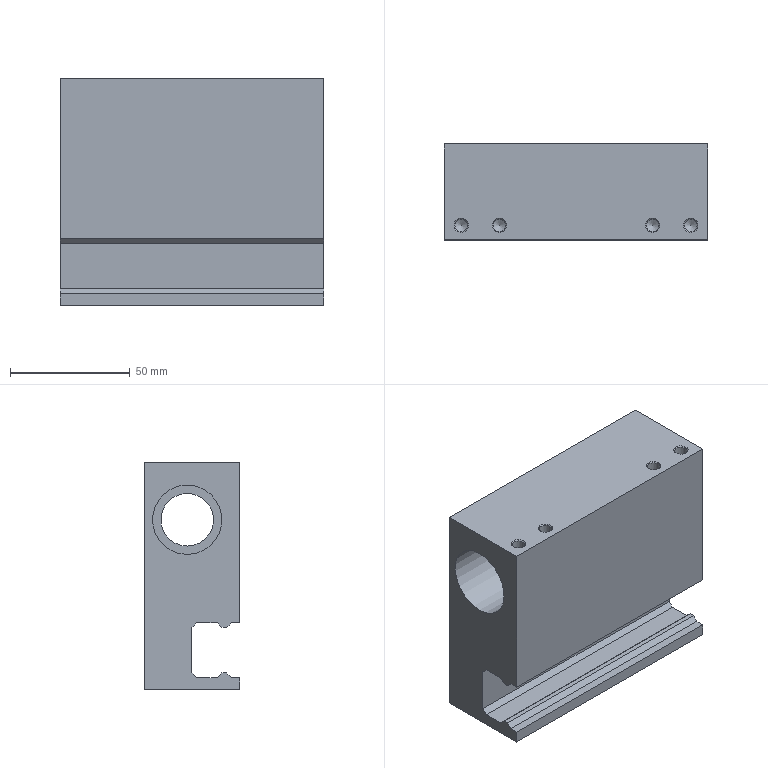Part | NX | features SIMPLE HOLE 10, SYMBOLIC_THREAD 9, DATUM_CSYS 5, HOLE PACKAGE 4, SKETCH 4, EXTRUDE 2, SUBTRACT 1 | 1 solid | 49 faces | box 110 x 40 x 95 mm | volume 307635 mm3 | plane 22 | cone 16 | cylinder 11 | commonest cylinder face diameters 5.2 x8 29 x2 22 x1
STEP:
#1=CARTESIAN_POINT('',(-55.,-3.5,11.5));
#2=VERTEX_POINT('',#1);
#3=CARTESIAN_POINT('',(55.,-3.5,11.5));
#4=VERTEX_POINT('',#3);
#5=CARTESIAN_POINT('',(55.,-3.5,11.5));
#6=DIRECTION('',(-1.,0.,0.));
#7=VECTOR('',#6,1000.);
#8=LINE('',#5,#7);
#9=EDGE_CURVE('',#2,#4,#8,.F.);
#10=ORIENTED_EDGE('',*,*,#9,.T.);
#11=CARTESIAN_POINT('',(55.,-3.5,78.5));
#12=VERTEX_POINT('',#11);
#13=CARTESIAN_POINT('',(55.,-3.5,78.5));
#14=DIRECTION('',(0.,0.,-1.));
#15=VECTOR('',#14,1000.);
#16=LINE('',#13,#15);
#17=EDGE_CURVE('',#12,#4,#16,.T.);
#18=ORIENTED_EDGE('',*,*,#17,.F.);
#19=CARTESIAN_POINT('',(-55.,-3.5,78.5));
#20=VERTEX_POINT('',#19);
#21=CARTESIAN_POINT('',(55.,-3.5,78.5));
#22=DIRECTION('',(-1.,0.,0.));
#23=VECTOR('',#22,1000.);
#24=LINE('',#21,#23);
#25=EDGE_CURVE('',#12,#20,#24,.T.);
#26=ORIENTED_EDGE('',*,*,#25,.T.);
#27=CARTESIAN_POINT('',(-55.,-3.5,78.5));
#28=DIRECTION('',(0.,0.,-1.));
#29=VECTOR('',#28,1000.);
#30=LINE('',#27,#29);
#31=EDGE_CURVE('',#20,#2,#30,.T.);
#32=ORIENTED_EDGE('',*,*,#31,.T.);
#33=EDGE_LOOP('',(#10,#18,#26,#32));
#34=FACE_BOUND('',#33,.T.);
#35=CARTESIAN_POINT('',(55.,-3.5,78.5));
#36=DIRECTION('',(0.,1.,0.));
#37=DIRECTION('',(0.,0.,1.));
#38=AXIS2_PLACEMENT_3D('',#35,#36,#37);
#39=PLANE('',#38);
#40=ADVANCED_FACE('',(#34),#39,.F.);
#41=CARTESIAN_POINT('',(55.,-3.5,-11.5));
#42=VERTEX_POINT('',#41);
#43=CARTESIAN_POINT('',(-55.,-3.5,-11.5));
#44=VERTEX_POINT('',#43);
#45=CARTESIAN_POINT('',(55.,-3.5,-11.5));
#46=DIRECTION('',(1.,0.,0.));
#47=VECTOR('',#46,1000.);
#48=LINE('',#45,#47);
#49=EDGE_CURVE('',#42,#44,#48,.F.);
#50=ORIENTED_EDGE('',*,*,#49,.T.);
#51=CARTESIAN_POINT('',(-55.,-3.5,-16.5));
#52=VERTEX_POINT('',#51);
#53=CARTESIAN_POINT('',(-55.,-3.5,78.5));
#54=DIRECTION('',(0.,0.,-1.));
#55=VECTOR('',#54,1000.);
#56=LINE('',#53,#55);
#57=EDGE_CURVE('',#44,#52,#56,.T.);
#58=ORIENTED_EDGE('',*,*,#57,.T.);
#59=CARTESIAN_POINT('',(55.,-3.5,-16.5));
#60=VERTEX_POINT('',#59);
#61=CARTESIAN_POINT('',(55.,-3.5,-16.5));
#62=DIRECTION('',(-1.,0.,0.));
#63=VECTOR('',#62,1000.);
#64=LINE('',#61,#63);
#65=EDGE_CURVE('',#60,#52,#64,.T.);
#66=ORIENTED_EDGE('',*,*,#65,.F.);
#67=CARTESIAN_POINT('',(55.,-3.5,78.5));
#68=DIRECTION('',(0.,0.,-1.));
#69=VECTOR('',#68,1000.);
#70=LINE('',#67,#69);
#71=EDGE_CURVE('',#42,#60,#70,.T.);
#72=ORIENTED_EDGE('',*,*,#71,.F.);
#73=EDGE_LOOP('',(#50,#58,#66,#72));
#74=FACE_BOUND('',#73,.T.);
#75=CARTESIAN_POINT('',(55.,-3.5,78.5));
#76=DIRECTION('',(0.,1.,0.));
#77=DIRECTION('',(0.,0.,1.));
#78=AXIS2_PLACEMENT_3D('',#75,#76,#77);
#79=PLANE('',#78);
#80=ADVANCED_FACE('',(#74),#79,.F.);
#81=CARTESIAN_POINT('',(55.,18.5,69.));
#82=VERTEX_POINT('',#81);
#83=CARTESIAN_POINT('',(55.,18.5,54.5));
#84=DIRECTION('',(-1.,0.,0.));
#85=DIRECTION('',(0.,0.,1.));
#86=AXIS2_PLACEMENT_3D('',#83,#84,#85);
#87=CIRCLE('',#86,14.5);
#88=EDGE_CURVE('',#82,#82,#87,.T.);
#89=ORIENTED_EDGE('',*,*,#88,.T.);
#90=EDGE_LOOP('',(#89));
#91=FACE_BOUND('',#90,.T.);
#92=ORIENTED_EDGE('',*,*,#17,.T.);
#93=CARTESIAN_POINT('',(55.,0.,11.5));
#94=VERTEX_POINT('',#93);
#95=CARTESIAN_POINT('',(55.,18.5,11.5));
#96=DIRECTION('',(0.,1.,0.));
#97=VECTOR('',#96,1000.);
#98=LINE('',#95,#97);
#99=EDGE_CURVE('',#94,#4,#98,.F.);
#100=ORIENTED_EDGE('',*,*,#99,.F.);
#101=CARTESIAN_POINT('',(55.,2.,9.5));
#102=VERTEX_POINT('',#101);
#103=CARTESIAN_POINT('',(55.,-12.25,23.75));
#104=DIRECTION('',(0.,0.7071,-0.7071));
#105=VECTOR('',#104,1000.);
#106=LINE('',#103,#105);
#107=EDGE_CURVE('',#102,#94,#106,.F.);
#108=ORIENTED_EDGE('',*,*,#107,.F.);
#109=CARTESIAN_POINT('',(55.,4.,9.5));
#110=VERTEX_POINT('',#109);
#111=CARTESIAN_POINT('',(55.,18.5,9.5));
#112=DIRECTION('',(0.,1.,0.));
#113=VECTOR('',#112,1000.);
#114=LINE('',#111,#113);
#115=EDGE_CURVE('',#110,#102,#114,.F.);
#116=ORIENTED_EDGE('',*,*,#115,.F.);
#117=CARTESIAN_POINT('',(55.,6.,11.5));
#118=VERTEX_POINT('',#117);
#119=CARTESIAN_POINT('',(55.,33.75,39.25));
#120=DIRECTION('',(0.,0.7071,0.7071));
#121=VECTOR('',#120,1000.);
#122=LINE('',#119,#121);
#123=EDGE_CURVE('',#118,#110,#122,.F.);
#124=ORIENTED_EDGE('',*,*,#123,.F.);
#125=CARTESIAN_POINT('',(55.,14.5,11.5));
#126=VERTEX_POINT('',#125);
#127=CARTESIAN_POINT('',(55.,18.5,11.5));
#128=DIRECTION('',(0.,1.,0.));
#129=VECTOR('',#128,1000.);
#130=LINE('',#127,#129);
#131=EDGE_CURVE('',#126,#118,#130,.F.);
#132=ORIENTED_EDGE('',*,*,#131,.F.);
#133=CARTESIAN_POINT('',(55.,16.5,9.5));
#134=VERTEX_POINT('',#133);
#135=CARTESIAN_POINT('',(55.,-5.,31.));
#136=DIRECTION('',(0.,0.7071,-0.7071));
#137=VECTOR('',#136,1000.);
#138=LINE('',#135,#137);
#139=EDGE_CURVE('',#134,#126,#138,.F.);
#140=ORIENTED_EDGE('',*,*,#139,.F.);
#141=CARTESIAN_POINT('',(55.,16.5,-9.5));
#142=VERTEX_POINT('',#141);
#143=CARTESIAN_POINT('',(55.,16.5,54.5));
#144=DIRECTION('',(0.,0.,-1.));
#145=VECTOR('',#144,1000.);
#146=LINE('',#143,#145);
#147=EDGE_CURVE('',#142,#134,#146,.F.);
#148=ORIENTED_EDGE('',*,*,#147,.F.);
#149=CARTESIAN_POINT('',(55.,14.5,-11.5));
#150=VERTEX_POINT('',#149);
#151=CARTESIAN_POINT('',(55.,49.5,23.5));
#152=DIRECTION('',(0.,-0.7071,-0.7071));
#153=VECTOR('',#152,1000.);
#154=LINE('',#151,#153);
#155=EDGE_CURVE('',#150,#142,#154,.F.);
#156=ORIENTED_EDGE('',*,*,#155,.F.);
#157=CARTESIAN_POINT('',(55.,6.,-11.5));
#158=VERTEX_POINT('',#157);
#159=CARTESIAN_POINT('',(55.,18.5,-11.5));
#160=DIRECTION('',(0.,-1.,0.));
#161=VECTOR('',#160,1000.);
#162=LINE('',#159,#161);
#163=EDGE_CURVE('',#158,#150,#162,.F.);
#164=ORIENTED_EDGE('',*,*,#163,.F.);
#165=CARTESIAN_POINT('',(55.,4.,-9.5));
#166=VERTEX_POINT('',#165);
#167=CARTESIAN_POINT('',(55.,-20.75,15.25));
#168=DIRECTION('',(0.,-0.7071,0.7071));
#169=VECTOR('',#168,1000.);
#170=LINE('',#167,#169);
#171=EDGE_CURVE('',#166,#158,#170,.F.);
#172=ORIENTED_EDGE('',*,*,#171,.F.);
#173=CARTESIAN_POINT('',(55.,2.,-9.5));
#174=VERTEX_POINT('',#173);
#175=CARTESIAN_POINT('',(55.,18.5,-9.5));
#176=DIRECTION('',(0.,-1.,0.));
#177=VECTOR('',#176,1000.);
#178=LINE('',#175,#177);
#179=EDGE_CURVE('',#174,#166,#178,.F.);
#180=ORIENTED_EDGE('',*,*,#179,.F.);
#181=CARTESIAN_POINT('',(55.,0.,-11.5));
#182=VERTEX_POINT('',#181);
#183=CARTESIAN_POINT('',(55.,42.25,30.75));
#184=DIRECTION('',(0.,-0.7071,-0.7071));
#185=VECTOR('',#184,1000.);
#186=LINE('',#183,#185);
#187=EDGE_CURVE('',#182,#174,#186,.F.);
#188=ORIENTED_EDGE('',*,*,#187,.F.);
#189=CARTESIAN_POINT('',(55.,18.5,-11.5));
#190=DIRECTION('',(0.,-1.,0.));
#191=VECTOR('',#190,1000.);
#192=LINE('',#189,#191);
#193=EDGE_CURVE('',#42,#182,#192,.F.);
#194=ORIENTED_EDGE('',*,*,#193,.F.);
#195=ORIENTED_EDGE('',*,*,#71,.T.);
#196=CARTESIAN_POINT('',(55.,36.5,-16.5));
#197=VERTEX_POINT('',#196);
#198=CARTESIAN_POINT('',(55.,-3.5,-16.5));
#199=DIRECTION('',(0.,1.,0.));
#200=VECTOR('',#199,1000.);
#201=LINE('',#198,#200);
#202=EDGE_CURVE('',#60,#197,#201,.T.);
#203=ORIENTED_EDGE('',*,*,#202,.T.);
#204=CARTESIAN_POINT('',(55.,36.5,78.5));
#205=VERTEX_POINT('',#204);
#206=CARTESIAN_POINT('',(55.,36.5,-16.5));
#207=DIRECTION('',(0.,0.,1.));
#208=VECTOR('',#207,1000.);
#209=LINE('',#206,#208);
#210=EDGE_CURVE('',#197,#205,#209,.T.);
#211=ORIENTED_EDGE('',*,*,#210,.T.);
#212=CARTESIAN_POINT('',(55.,36.5,78.5));
#213=DIRECTION('',(0.,-1.,0.));
#214=VECTOR('',#213,1000.);
#215=LINE('',#212,#214);
#216=EDGE_CURVE('',#205,#12,#215,.T.);
#217=ORIENTED_EDGE('',*,*,#216,.T.);
#218=EDGE_LOOP('',(#92,#100,#108,#116,#124,#132,#140,#148,#156,#164,#172,#180,#188,#194,#195,#203,#211,#217));
#219=FACE_BOUND('',#218,.T.);
#220=CARTESIAN_POINT('',(55.,18.5,54.5));
#221=DIRECTION('',(1.,0.,0.));
#222=DIRECTION('',(0.,0.,-1.));
#223=AXIS2_PLACEMENT_3D('',#220,#221,#222);
#224=PLANE('',#223);
#225=ADVANCED_FACE('',(#91,#219),#224,.T.);
#226=CARTESIAN_POINT('',(-55.,18.5,40.));
#227=VERTEX_POINT('',#226);
#228=CARTESIAN_POINT('',(-55.,18.5,54.5));
#229=DIRECTION('',(1.,0.,0.));
#230=DIRECTION('',(0.,0.,-1.));
#231=AXIS2_PLACEMENT_3D('',#228,#229,#230);
#232=CIRCLE('',#231,14.5);
#233=EDGE_CURVE('',#227,#227,#232,.T.);
#234=ORIENTED_EDGE('',*,*,#233,.T.);
#235=EDGE_LOOP('',(#234));
#236=FACE_BOUND('',#235,.T.);
#237=CARTESIAN_POINT('',(-55.,0.,11.5));
#238=VERTEX_POINT('',#237);
#239=CARTESIAN_POINT('',(-55.,18.5,11.5));
#240=DIRECTION('',(0.,1.,0.));
#241=VECTOR('',#240,1000.);
#242=LINE('',#239,#241);
#243=EDGE_CURVE('',#238,#2,#242,.F.);
#244=ORIENTED_EDGE('',*,*,#243,.T.);
#245=ORIENTED_EDGE('',*,*,#31,.F.);
#246=CARTESIAN_POINT('',(-55.,36.5,78.5));
#247=VERTEX_POINT('',#246);
#248=CARTESIAN_POINT('',(-55.,36.5,78.5));
#249=DIRECTION('',(0.,-1.,0.));
#250=VECTOR('',#249,1000.);
#251=LINE('',#248,#250);
#252=EDGE_CURVE('',#247,#20,#251,.T.);
#253=ORIENTED_EDGE('',*,*,#252,.F.);
#254=CARTESIAN_POINT('',(-55.,36.5,-16.5));
#255=VERTEX_POINT('',#254);
#256=CARTESIAN_POINT('',(-55.,36.5,-16.5));
#257=DIRECTION('',(0.,0.,1.));
#258=VECTOR('',#257,1000.);
#259=LINE('',#256,#258);
#260=EDGE_CURVE('',#255,#247,#259,.T.);
#261=ORIENTED_EDGE('',*,*,#260,.F.);
#262=CARTESIAN_POINT('',(-55.,-3.5,-16.5));
#263=DIRECTION('',(0.,1.,0.));
#264=VECTOR('',#263,1000.);
#265=LINE('',#262,#264);
#266=EDGE_CURVE('',#52,#255,#265,.T.);
#267=ORIENTED_EDGE('',*,*,#266,.F.);
#268=ORIENTED_EDGE('',*,*,#57,.F.);
#269=CARTESIAN_POINT('',(-55.,0.,-11.5));
#270=VERTEX_POINT('',#269);
#271=CARTESIAN_POINT('',(-55.,18.5,-11.5));
#272=DIRECTION('',(0.,-1.,0.));
#273=VECTOR('',#272,1000.);
#274=LINE('',#271,#273);
#275=EDGE_CURVE('',#44,#270,#274,.F.);
#276=ORIENTED_EDGE('',*,*,#275,.T.);
#277=CARTESIAN_POINT('',(-55.,2.,-9.5));
#278=VERTEX_POINT('',#277);
#279=CARTESIAN_POINT('',(-55.,42.25,30.75));
#280=DIRECTION('',(0.,-0.7071,-0.7071));
#281=VECTOR('',#280,1000.);
#282=LINE('',#279,#281);
#283=EDGE_CURVE('',#270,#278,#282,.F.);
#284=ORIENTED_EDGE('',*,*,#283,.T.);
#285=CARTESIAN_POINT('',(-55.,4.,-9.5));
#286=VERTEX_POINT('',#285);
#287=CARTESIAN_POINT('',(-55.,18.5,-9.5));
#288=DIRECTION('',(0.,-1.,0.));
#289=VECTOR('',#288,1000.);
#290=LINE('',#287,#289);
#291=EDGE_CURVE('',#278,#286,#290,.F.);
#292=ORIENTED_EDGE('',*,*,#291,.T.);
#293=CARTESIAN_POINT('',(-55.,6.,-11.5));
#294=VERTEX_POINT('',#293);
#295=CARTESIAN_POINT('',(-55.,-20.75,15.25));
#296=DIRECTION('',(0.,-0.7071,0.7071));
#297=VECTOR('',#296,1000.);
#298=LINE('',#295,#297);
#299=EDGE_CURVE('',#286,#294,#298,.F.);
#300=ORIENTED_EDGE('',*,*,#299,.T.);
#301=CARTESIAN_POINT('',(-55.,14.5,-11.5));
#302=VERTEX_POINT('',#301);
#303=CARTESIAN_POINT('',(-55.,18.5,-11.5));
#304=DIRECTION('',(0.,-1.,0.));
#305=VECTOR('',#304,1000.);
#306=LINE('',#303,#305);
#307=EDGE_CURVE('',#294,#302,#306,.F.);
#308=ORIENTED_EDGE('',*,*,#307,.T.);
#309=CARTESIAN_POINT('',(-55.,16.5,-9.5));
#310=VERTEX_POINT('',#309);
#311=CARTESIAN_POINT('',(-55.,49.5,23.5));
#312=DIRECTION('',(0.,-0.7071,-0.7071));
#313=VECTOR('',#312,1000.);
#314=LINE('',#311,#313);
#315=EDGE_CURVE('',#302,#310,#314,.F.);
#316=ORIENTED_EDGE('',*,*,#315,.T.);
#317=CARTESIAN_POINT('',(-55.,16.5,9.5));
#318=VERTEX_POINT('',#317);
#319=CARTESIAN_POINT('',(-55.,16.5,54.5));
#320=DIRECTION('',(0.,0.,-1.));
#321=VECTOR('',#320,1000.);
#322=LINE('',#319,#321);
#323=EDGE_CURVE('',#310,#318,#322,.F.);
#324=ORIENTED_EDGE('',*,*,#323,.T.);
#325=CARTESIAN_POINT('',(-55.,14.5,11.5));
#326=VERTEX_POINT('',#325);
#327=CARTESIAN_POINT('',(-55.,-5.,31.));
#328=DIRECTION('',(0.,0.7071,-0.7071));
#329=VECTOR('',#328,1000.);
#330=LINE('',#327,#329);
#331=EDGE_CURVE('',#318,#326,#330,.F.);
#332=ORIENTED_EDGE('',*,*,#331,.T.);
#333=CARTESIAN_POINT('',(-55.,6.,11.5));
#334=VERTEX_POINT('',#333);
#335=CARTESIAN_POINT('',(-55.,18.5,11.5));
#336=DIRECTION('',(0.,1.,0.));
#337=VECTOR('',#336,1000.);
#338=LINE('',#335,#337);
#339=EDGE_CURVE('',#326,#334,#338,.F.);
#340=ORIENTED_EDGE('',*,*,#339,.T.);
#341=CARTESIAN_POINT('',(-55.,4.,9.5));
#342=VERTEX_POINT('',#341);
#343=CARTESIAN_POINT('',(-55.,33.75,39.25));
#344=DIRECTION('',(0.,0.7071,0.7071));
#345=VECTOR('',#344,1000.);
#346=LINE('',#343,#345);
#347=EDGE_CURVE('',#334,#342,#346,.F.);
#348=ORIENTED_EDGE('',*,*,#347,.T.);
#349=CARTESIAN_POINT('',(-55.,2.,9.5));
#350=VERTEX_POINT('',#349);
#351=CARTESIAN_POINT('',(-55.,18.5,9.5));
#352=DIRECTION('',(0.,1.,0.));
#353=VECTOR('',#352,1000.);
#354=LINE('',#351,#353);
#355=EDGE_CURVE('',#342,#350,#354,.F.);
#356=ORIENTED_EDGE('',*,*,#355,.T.);
#357=CARTESIAN_POINT('',(-55.,-12.25,23.75));
#358=DIRECTION('',(0.,0.7071,-0.7071));
#359=VECTOR('',#358,1000.);
#360=LINE('',#357,#359);
#361=EDGE_CURVE('',#350,#238,#360,.F.);
#362=ORIENTED_EDGE('',*,*,#361,.T.);
#363=EDGE_LOOP('',(#244,#245,#253,#261,#267,#268,#276,#284,#292,#300,#308,#316,#324,#332,#340,#348,#356,#362));
#364=FACE_BOUND('',#363,.T.);
#365=CARTESIAN_POINT('',(-55.,18.5,54.5));
#366=DIRECTION('',(1.,0.,0.));
#367=DIRECTION('',(0.,0.,-1.));
#368=AXIS2_PLACEMENT_3D('',#365,#366,#367);
#369=PLANE('',#368);
#370=ADVANCED_FACE('',(#236,#364),#369,.F.);
#371=ORIENTED_EDGE('',*,*,#266,.T.);
#372=CARTESIAN_POINT('',(55.,36.5,-16.5));
#373=DIRECTION('',(-1.,0.,0.));
#374=VECTOR('',#373,1000.);
#375=LINE('',#372,#374);
#376=EDGE_CURVE('',#197,#255,#375,.T.);
#377=ORIENTED_EDGE('',*,*,#376,.F.);
#378=ORIENTED_EDGE('',*,*,#202,.F.);
#379=ORIENTED_EDGE('',*,*,#65,.T.);
#380=EDGE_LOOP('',(#371,#377,#378,#379));
#381=FACE_BOUND('',#380,.T.);
#382=CARTESIAN_POINT('',(55.,-3.5,-16.5));
#383=DIRECTION('',(0.,0.,1.));
#384=DIRECTION('',(1.,0.,0.));
#385=AXIS2_PLACEMENT_3D('',#382,#383,#384);
#386=PLANE('',#385);
#387=ADVANCED_FACE('',(#381),#386,.F.);
#388=CARTESIAN_POINT('',(-46.,36.5,33.5));
#389=VERTEX_POINT('',#388);
#390=CARTESIAN_POINT('',(-46.,36.5,36.5));
#391=DIRECTION('',(0.,-1.,0.));
#392=DIRECTION('',(0.,0.,-1.));
#393=AXIS2_PLACEMENT_3D('',#390,#391,#392);
#394=CIRCLE('',#393,3.);
#395=EDGE_CURVE('',#389,#389,#394,.T.);
#396=ORIENTED_EDGE('',*,*,#395,.T.);
#397=EDGE_LOOP('',(#396));
#398=FACE_BOUND('',#397,.T.);
#399=CARTESIAN_POINT('',(-46.,36.5,17.5));
#400=VERTEX_POINT('',#399);
#401=CARTESIAN_POINT('',(-46.,36.5,20.5));
#402=DIRECTION('',(0.,-1.,0.));
#403=DIRECTION('',(0.,0.,-1.));
#404=AXIS2_PLACEMENT_3D('',#401,#402,#403);
#405=CIRCLE('',#404,3.);
#406=EDGE_CURVE('',#400,#400,#405,.T.);
#407=ORIENTED_EDGE('',*,*,#406,.T.);
#408=EDGE_LOOP('',(#407));
#409=FACE_BOUND('',#408,.T.);
#410=CARTESIAN_POINT('',(16.,36.5,17.5));
#411=VERTEX_POINT('',#410);
#412=CARTESIAN_POINT('',(16.,36.5,20.5));
#413=DIRECTION('',(0.,-1.,0.));
#414=DIRECTION('',(0.,0.,-1.));
#415=AXIS2_PLACEMENT_3D('',#412,#413,#414);
#416=CIRCLE('',#415,3.);
#417=EDGE_CURVE('',#411,#411,#416,.T.);
#418=ORIENTED_EDGE('',*,*,#417,.T.);
#419=EDGE_LOOP('',(#418));
#420=FACE_BOUND('',#419,.T.);
#421=CARTESIAN_POINT('',(16.,36.5,33.5));
#422=VERTEX_POINT('',#421);
#423=CARTESIAN_POINT('',(16.,36.5,36.5));
#424=DIRECTION('',(0.,-1.,0.));
#425=DIRECTION('',(0.,0.,-1.));
#426=AXIS2_PLACEMENT_3D('',#423,#424,#425);
#427=CIRCLE('',#426,3.);
#428=EDGE_CURVE('',#422,#422,#427,.T.);
#429=ORIENTED_EDGE('',*,*,#428,.T.);
#430=EDGE_LOOP('',(#429));
#431=FACE_BOUND('',#430,.T.);
#432=ORIENTED_EDGE('',*,*,#260,.T.);
#433=CARTESIAN_POINT('',(55.,36.5,78.5));
#434=DIRECTION('',(-1.,0.,0.));
#435=VECTOR('',#434,1000.);
#436=LINE('',#433,#435);
#437=EDGE_CURVE('',#205,#247,#436,.T.);
#438=ORIENTED_EDGE('',*,*,#437,.F.);
#439=ORIENTED_EDGE('',*,*,#210,.F.);
#440=ORIENTED_EDGE('',*,*,#376,.T.);
#441=EDGE_LOOP('',(#432,#438,#439,#440));
#442=FACE_BOUND('',#441,.T.);
#443=CARTESIAN_POINT('',(55.,36.5,-16.5));
#444=DIRECTION('',(0.,-1.,0.));
#445=DIRECTION('',(0.,0.,-1.));
#446=AXIS2_PLACEMENT_3D('',#443,#444,#445);
#447=PLANE('',#446);
#448=ADVANCED_FACE('',(#398,#409,#420,#431,#442),#447,.F.);
#449=CARTESIAN_POINT('',(45.,2.5,78.5));
#450=VERTEX_POINT('',#449);
#451=CARTESIAN_POINT('',(48.,2.5,78.5));
#452=DIRECTION('',(0.,0.,-1.));
#453=DIRECTION('',(-1.,0.,0.));
#454=AXIS2_PLACEMENT_3D('',#451,#452,#453);
#455=CIRCLE('',#454,3.);
#456=EDGE_CURVE('',#450,#450,#455,.T.);
#457=ORIENTED_EDGE('',*,*,#456,.T.);
#458=EDGE_LOOP('',(#457));
#459=FACE_BOUND('',#458,.T.);
#460=CARTESIAN_POINT('',(29.,2.5,78.5));
#461=VERTEX_POINT('',#460);
#462=CARTESIAN_POINT('',(32.,2.5,78.5));
#463=DIRECTION('',(0.,0.,-1.));
#464=DIRECTION('',(-1.,0.,0.));
#465=AXIS2_PLACEMENT_3D('',#462,#463,#464);
#466=CIRCLE('',#465,3.);
#467=EDGE_CURVE('',#461,#461,#466,.T.);
#468=ORIENTED_EDGE('',*,*,#467,.T.);
#469=EDGE_LOOP('',(#468));
#470=FACE_BOUND('',#469,.T.);
#471=CARTESIAN_POINT('',(-35.,2.5,78.5));
#472=VERTEX_POINT('',#471);
#473=CARTESIAN_POINT('',(-32.,2.5,78.5));
#474=DIRECTION('',(0.,0.,-1.));
#475=DIRECTION('',(-1.,0.,0.));
#476=AXIS2_PLACEMENT_3D('',#473,#474,#475);
#477=CIRCLE('',#476,3.);
#478=EDGE_CURVE('',#472,#472,#477,.T.);
#479=ORIENTED_EDGE('',*,*,#478,.T.);
#480=EDGE_LOOP('',(#479));
#481=FACE_BOUND('',#480,.T.);
#482=CARTESIAN_POINT('',(-51.,2.5,78.5));
#483=VERTEX_POINT('',#482);
#484=CARTESIAN_POINT('',(-48.,2.5,78.5));
#485=DIRECTION('',(0.,0.,-1.));
#486=DIRECTION('',(-1.,0.,0.));
#487=AXIS2_PLACEMENT_3D('',#484,#485,#486);
#488=CIRCLE('',#487,3.);
#489=EDGE_CURVE('',#483,#483,#488,.T.);
#490=ORIENTED_EDGE('',*,*,#489,.T.);
#491=EDGE_LOOP('',(#490));
#492=FACE_BOUND('',#491,.T.);
#493=ORIENTED_EDGE('',*,*,#252,.T.);
#494=ORIENTED_EDGE('',*,*,#25,.F.);
#495=ORIENTED_EDGE('',*,*,#216,.F.);
#496=ORIENTED_EDGE('',*,*,#437,.T.);
#497=EDGE_LOOP('',(#493,#494,#495,#496));
#498=FACE_BOUND('',#497,.T.);
#499=CARTESIAN_POINT('',(55.,36.5,78.5));
#500=DIRECTION('',(0.,0.,-1.));
#501=DIRECTION('',(-1.,0.,0.));
#502=AXIS2_PLACEMENT_3D('',#499,#500,#501);
#503=PLANE('',#502);
#504=ADVANCED_FACE('',(#459,#470,#481,#492,#498),#503,.F.);
#505=CARTESIAN_POINT('',(25.,18.5,65.5));
#506=VERTEX_POINT('',#505);
#507=CARTESIAN_POINT('',(25.,18.5,54.5));
#508=DIRECTION('',(-1.,0.,0.));
#509=DIRECTION('',(0.,0.,1.));
#510=AXIS2_PLACEMENT_3D('',#507,#508,#509);
#511=CIRCLE('',#510,11.);
#512=EDGE_CURVE('',#506,#506,#511,.T.);
#513=ORIENTED_EDGE('',*,*,#512,.F.);
#514=EDGE_LOOP('',(#513));
#515=FACE_BOUND('',#514,.T.);
#516=CARTESIAN_POINT('',(-25.,18.5,43.5));
#517=VERTEX_POINT('',#516);
#518=CARTESIAN_POINT('',(-25.,18.5,54.5));
#519=DIRECTION('',(1.,0.,0.));
#520=DIRECTION('',(0.,0.,-1.));
#521=AXIS2_PLACEMENT_3D('',#518,#519,#520);
#522=CIRCLE('',#521,11.);
#523=EDGE_CURVE('',#517,#517,#522,.T.);
#524=ORIENTED_EDGE('',*,*,#523,.F.);
#525=EDGE_LOOP('',(#524));
#526=FACE_BOUND('',#525,.T.);
#527=CARTESIAN_POINT('',(55.,18.5,54.5));
#528=DIRECTION('',(-1.,0.,0.));
#529=DIRECTION('',(0.,0.,1.));
#530=AXIS2_PLACEMENT_3D('',#527,#528,#529);
#531=CYLINDRICAL_SURFACE('',#530,11.);
#532=ADVANCED_FACE('',(#515,#526),#531,.F.);
#533=CARTESIAN_POINT('',(225.,2.,-9.5));
#534=DIRECTION('',(-1.,0.,0.));
#535=VECTOR('',#534,1000.);
#536=LINE('',#533,#535);
#537=EDGE_CURVE('',#278,#174,#536,.F.);
#538=ORIENTED_EDGE('',*,*,#537,.F.);
#539=ORIENTED_EDGE('',*,*,#283,.F.);
#540=CARTESIAN_POINT('',(225.,0.,-11.5));
#541=DIRECTION('',(-1.,0.,0.));
#542=VECTOR('',#541,1000.);
#543=LINE('',#540,#542);
#544=EDGE_CURVE('',#270,#182,#543,.F.);
#545=ORIENTED_EDGE('',*,*,#544,.T.);
#546=ORIENTED_EDGE('',*,*,#187,.T.);
#547=EDGE_LOOP('',(#538,#539,#545,#546));
#548=FACE_BOUND('',#547,.T.);
#549=CARTESIAN_POINT('',(225.,0.,-11.5));
#550=DIRECTION('',(0.,-0.7071,0.7071));
#551=DIRECTION('',(0.,-0.7071,-0.7071));
#552=AXIS2_PLACEMENT_3D('',#549,#550,#551);
#553=PLANE('',#552);
#554=ADVANCED_FACE('',(#548),#553,.T.);
#555=CARTESIAN_POINT('',(225.,4.,-9.5));
#556=DIRECTION('',(-1.,0.,0.));
#557=VECTOR('',#556,1000.);
#558=LINE('',#555,#557);
#559=EDGE_CURVE('',#286,#166,#558,.F.);
#560=ORIENTED_EDGE('',*,*,#559,.F.);
#561=ORIENTED_EDGE('',*,*,#291,.F.);
#562=ORIENTED_EDGE('',*,*,#537,.T.);
#563=ORIENTED_EDGE('',*,*,#179,.T.);
#564=EDGE_LOOP('',(#560,#561,#562,#563));
#565=FACE_BOUND('',#564,.T.);
#566=CARTESIAN_POINT('',(225.,2.,-9.5));
#567=DIRECTION('',(0.,0.,1.));
#568=DIRECTION('',(1.,0.,0.));
#569=AXIS2_PLACEMENT_3D('',#566,#567,#568);
#570=PLANE('',#569);
#571=ADVANCED_FACE('',(#565),#570,.T.);
#572=CARTESIAN_POINT('',(225.,6.,-11.5));
#573=DIRECTION('',(-1.,0.,0.));
#574=VECTOR('',#573,1000.);
#575=LINE('',#572,#574);
#576=EDGE_CURVE('',#294,#158,#575,.F.);
#577=ORIENTED_EDGE('',*,*,#576,.F.);
#578=ORIENTED_EDGE('',*,*,#299,.F.);
#579=ORIENTED_EDGE('',*,*,#559,.T.);
#580=ORIENTED_EDGE('',*,*,#171,.T.);
#581=EDGE_LOOP('',(#577,#578,#579,#580));
#582=FACE_BOUND('',#581,.T.);
#583=CARTESIAN_POINT('',(225.,4.,-9.5));
#584=DIRECTION('',(0.,0.7071,0.7071));
#585=DIRECTION('',(0.,-0.7071,0.7071));
#586=AXIS2_PLACEMENT_3D('',#583,#584,#585);
#587=PLANE('',#586);
#588=ADVANCED_FACE('',(#582),#587,.T.);
#589=CARTESIAN_POINT('',(225.,14.5,-11.5));
#590=DIRECTION('',(-1.,0.,0.));
#591=VECTOR('',#590,1000.);
#592=LINE('',#589,#591);
#593=EDGE_CURVE('',#302,#150,#592,.F.);
#594=ORIENTED_EDGE('',*,*,#593,.F.);
#595=ORIENTED_EDGE('',*,*,#307,.F.);
#596=ORIENTED_EDGE('',*,*,#576,.T.);
#597=ORIENTED_EDGE('',*,*,#163,.T.);
#598=EDGE_LOOP('',(#594,#595,#596,#597));
#599=FACE_BOUND('',#598,.T.);
#600=CARTESIAN_POINT('',(225.,6.,-11.5));
#601=DIRECTION('',(0.,0.,1.));
#602=DIRECTION('',(0.,-1.,0.));
#603=AXIS2_PLACEMENT_3D('',#600,#601,#602);
#604=PLANE('',#603);
#605=ADVANCED_FACE('',(#599),#604,.T.);
#606=CARTESIAN_POINT('',(225.,16.5,-9.5));
#607=DIRECTION('',(-1.,0.,0.));
#608=VECTOR('',#607,1000.);
#609=LINE('',#606,#608);
#610=EDGE_CURVE('',#310,#142,#609,.F.);
#611=ORIENTED_EDGE('',*,*,#610,.F.);
#612=ORIENTED_EDGE('',*,*,#315,.F.);
#613=ORIENTED_EDGE('',*,*,#593,.T.);
#614=ORIENTED_EDGE('',*,*,#155,.T.);
#615=EDGE_LOOP('',(#611,#612,#613,#614));
#616=FACE_BOUND('',#615,.T.);
#617=CARTESIAN_POINT('',(225.,14.5,-11.5));
#618=DIRECTION('',(0.,-0.7071,0.7071));
#619=DIRECTION('',(0.,-0.7071,-0.7071));
#620=AXIS2_PLACEMENT_3D('',#617,#618,#619);
#621=PLANE('',#620);
#622=ADVANCED_FACE('',(#616),#621,.T.);
#623=CARTESIAN_POINT('',(225.,16.5,9.5));
#624=DIRECTION('',(-1.,0.,0.));
#625=VECTOR('',#624,1000.);
#626=LINE('',#623,#625);
#627=EDGE_CURVE('',#318,#134,#626,.F.);
#628=ORIENTED_EDGE('',*,*,#627,.F.);
#629=ORIENTED_EDGE('',*,*,#323,.F.);
#630=ORIENTED_EDGE('',*,*,#610,.T.);
#631=ORIENTED_EDGE('',*,*,#147,.T.);
#632=EDGE_LOOP('',(#628,#629,#630,#631));
#633=FACE_BOUND('',#632,.T.);
#634=CARTESIAN_POINT('',(225.,16.5,0.));
#635=DIRECTION('',(0.,-1.,0.));
#636=DIRECTION('',(0.,0.,-1.));
#637=AXIS2_PLACEMENT_3D('',#634,#635,#636);
#638=PLANE('',#637);
#639=ADVANCED_FACE('',(#633),#638,.T.);
#640=CARTESIAN_POINT('',(225.,14.5,11.5));
#641=DIRECTION('',(-1.,0.,0.));
#642=VECTOR('',#641,1000.);
#643=LINE('',#640,#642);
#644=EDGE_CURVE('',#326,#126,#643,.F.);
#645=ORIENTED_EDGE('',*,*,#644,.F.);
#646=ORIENTED_EDGE('',*,*,#331,.F.);
#647=ORIENTED_EDGE('',*,*,#627,.T.);
#648=ORIENTED_EDGE('',*,*,#139,.T.);
#649=EDGE_LOOP('',(#645,#646,#647,#648));
#650=FACE_BOUND('',#649,.T.);
#651=CARTESIAN_POINT('',(225.,16.5,9.5));
#652=DIRECTION('',(0.,-0.7071,-0.7071));
#653=DIRECTION('',(0.,0.7071,-0.7071));
#654=AXIS2_PLACEMENT_3D('',#651,#652,#653);
#655=PLANE('',#654);
#656=ADVANCED_FACE('',(#650),#655,.T.);
#657=CARTESIAN_POINT('',(225.,6.,11.5));
#658=DIRECTION('',(-1.,0.,0.));
#659=VECTOR('',#658,1000.);
#660=LINE('',#657,#659);
#661=EDGE_CURVE('',#334,#118,#660,.F.);
#662=ORIENTED_EDGE('',*,*,#661,.F.);
#663=ORIENTED_EDGE('',*,*,#339,.F.);
#664=ORIENTED_EDGE('',*,*,#644,.T.);
#665=ORIENTED_EDGE('',*,*,#131,.T.);
#666=EDGE_LOOP('',(#662,#663,#664,#665));
#667=FACE_BOUND('',#666,.T.);
#668=CARTESIAN_POINT('',(225.,14.5,11.5));
#669=DIRECTION('',(0.,0.,-1.));
#670=DIRECTION('',(0.,1.,0.));
#671=AXIS2_PLACEMENT_3D('',#668,#669,#670);
#672=PLANE('',#671);
#673=ADVANCED_FACE('',(#667),#672,.T.);
#674=CARTESIAN_POINT('',(225.,4.,9.5));
#675=DIRECTION('',(-1.,0.,0.));
#676=VECTOR('',#675,1000.);
#677=LINE('',#674,#676);
#678=EDGE_CURVE('',#342,#110,#677,.F.);
#679=ORIENTED_EDGE('',*,*,#678,.F.);
#680=ORIENTED_EDGE('',*,*,#347,.F.);
#681=ORIENTED_EDGE('',*,*,#661,.T.);
#682=ORIENTED_EDGE('',*,*,#123,.T.);
#683=EDGE_LOOP('',(#679,#680,#681,#682));
#684=FACE_BOUND('',#683,.T.);
#685=CARTESIAN_POINT('',(225.,6.,11.5));
#686=DIRECTION('',(0.,0.7071,-0.7071));
#687=DIRECTION('',(0.,0.7071,0.7071));
#688=AXIS2_PLACEMENT_3D('',#685,#686,#687);
#689=PLANE('',#688);
#690=ADVANCED_FACE('',(#684),#689,.T.);
#691=CARTESIAN_POINT('',(225.,2.,9.5));
#692=DIRECTION('',(-1.,0.,0.));
#693=VECTOR('',#692,1000.);
#694=LINE('',#691,#693);
#695=EDGE_CURVE('',#350,#102,#694,.F.);
#696=ORIENTED_EDGE('',*,*,#695,.F.);
#697=ORIENTED_EDGE('',*,*,#355,.F.);
#698=ORIENTED_EDGE('',*,*,#678,.T.);
#699=ORIENTED_EDGE('',*,*,#115,.T.);
#700=EDGE_LOOP('',(#696,#697,#698,#699));
#701=FACE_BOUND('',#700,.T.);
#702=CARTESIAN_POINT('',(225.,4.,9.5));
#703=DIRECTION('',(0.,0.,-1.));
#704=DIRECTION('',(-1.,0.,0.));
#705=AXIS2_PLACEMENT_3D('',#702,#703,#704);
#706=PLANE('',#705);
#707=ADVANCED_FACE('',(#701),#706,.T.);
#708=CARTESIAN_POINT('',(225.,0.,11.5));
#709=DIRECTION('',(-1.,0.,0.));
#710=VECTOR('',#709,1000.);
#711=LINE('',#708,#710);
#712=EDGE_CURVE('',#238,#94,#711,.F.);
#713=ORIENTED_EDGE('',*,*,#712,.F.);
#714=ORIENTED_EDGE('',*,*,#361,.F.);
#715=ORIENTED_EDGE('',*,*,#695,.T.);
#716=ORIENTED_EDGE('',*,*,#107,.T.);
#717=EDGE_LOOP('',(#713,#714,#715,#716));
#718=FACE_BOUND('',#717,.T.);
#719=CARTESIAN_POINT('',(225.,2.,9.5));
#720=DIRECTION('',(0.,-0.7071,-0.7071));
#721=DIRECTION('',(0.,0.7071,-0.7071));
#722=AXIS2_PLACEMENT_3D('',#719,#720,#721);
#723=PLANE('',#722);
#724=ADVANCED_FACE('',(#718),#723,.T.);
#725=ORIENTED_EDGE('',*,*,#9,.F.);
#726=ORIENTED_EDGE('',*,*,#243,.F.);
#727=ORIENTED_EDGE('',*,*,#712,.T.);
#728=ORIENTED_EDGE('',*,*,#99,.T.);
#729=EDGE_LOOP('',(#725,#726,#727,#728));
#730=FACE_BOUND('',#729,.T.);
#731=CARTESIAN_POINT('',(225.,0.,11.5));
#732=DIRECTION('',(0.,0.,-1.));
#733=DIRECTION('',(0.,1.,0.));
#734=AXIS2_PLACEMENT_3D('',#731,#732,#733);
#735=PLANE('',#734);
#736=ADVANCED_FACE('',(#730),#735,.T.);
#737=ORIENTED_EDGE('',*,*,#544,.F.);
#738=ORIENTED_EDGE('',*,*,#275,.F.);
#739=ORIENTED_EDGE('',*,*,#49,.F.);
#740=ORIENTED_EDGE('',*,*,#193,.T.);
#741=EDGE_LOOP('',(#737,#738,#739,#740));
#742=FACE_BOUND('',#741,.T.);
#743=CARTESIAN_POINT('',(225.,-5.5,-11.5));
#744=DIRECTION('',(0.,0.,1.));
#745=DIRECTION('',(0.,-1.,0.));
#746=AXIS2_PLACEMENT_3D('',#743,#744,#745);
#747=PLANE('',#746);
#748=ADVANCED_FACE('',(#742),#747,.T.);
#749=CARTESIAN_POINT('',(-50.6,2.5,60.5));
#750=VERTEX_POINT('',#749);
#751=CARTESIAN_POINT('',(-48.,2.5,60.5));
#752=DIRECTION('',(0.,0.,-1.));
#753=DIRECTION('',(-1.,0.,0.));
#754=AXIS2_PLACEMENT_3D('',#751,#752,#753);
#755=CIRCLE('',#754,2.6);
#756=EDGE_CURVE('',#750,#750,#755,.F.);
#757=ORIENTED_EDGE('',*,*,#756,.T.);
#758=EDGE_LOOP('',(#757));
#759=FACE_BOUND('',#758,.T.);
#760=CARTESIAN_POINT('',(-48.,2.5,58.938));
#761=VERTEX_POINT('',#760);
#762=VERTEX_LOOP('',#761);
#763=FACE_BOUND('',#762,.T.);
#764=CARTESIAN_POINT('',(-48.,2.5,60.5));
#765=DIRECTION('',(0.,0.,1.));
#766=DIRECTION('',(1.,0.,0.));
#767=AXIS2_PLACEMENT_3D('',#764,#765,#766);
#768=CONICAL_SURFACE('',#767,2.6,1.03);
#769=ADVANCED_FACE('',(#759,#763),#768,.F.);
#770=CARTESIAN_POINT('',(-50.6,2.5,78.1));
#771=VERTEX_POINT('',#770);
#772=CARTESIAN_POINT('',(-48.,2.5,78.1));
#773=DIRECTION('',(0.,0.,-1.));
#774=DIRECTION('',(-1.,0.,0.));
#775=AXIS2_PLACEMENT_3D('',#772,#773,#774);
#776=CIRCLE('',#775,2.6);
#777=EDGE_CURVE('',#771,#771,#776,.F.);
#778=ORIENTED_EDGE('',*,*,#777,.T.);
#779=EDGE_LOOP('',(#778));
#780=FACE_BOUND('',#779,.T.);
#781=ORIENTED_EDGE('',*,*,#756,.F.);
#782=EDGE_LOOP('',(#781));
#783=FACE_BOUND('',#782,.T.);
#784=CARTESIAN_POINT('',(-48.,2.5,78.5));
#785=DIRECTION('',(0.,0.,-1.));
#786=DIRECTION('',(-1.,0.,0.));
#787=AXIS2_PLACEMENT_3D('',#784,#785,#786);
#788=CYLINDRICAL_SURFACE('',#787,2.6);
#789=ADVANCED_FACE('',(#780,#783),#788,.F.);
#790=ORIENTED_EDGE('',*,*,#777,.F.);
#791=EDGE_LOOP('',(#790));
#792=FACE_BOUND('',#791,.T.);
#793=ORIENTED_EDGE('',*,*,#489,.F.);
#794=EDGE_LOOP('',(#793));
#795=FACE_BOUND('',#794,.T.);
#796=CARTESIAN_POINT('',(-48.,2.5,78.5));
#797=DIRECTION('',(0.,0.,1.));
#798=DIRECTION('',(1.,0.,0.));
#799=AXIS2_PLACEMENT_3D('',#796,#797,#798);
#800=CONICAL_SURFACE('',#799,3.,0.7854);
#801=ADVANCED_FACE('',(#792,#795),#800,.F.);
#802=CARTESIAN_POINT('',(-34.6,2.5,60.5));
#803=VERTEX_POINT('',#802);
#804=CARTESIAN_POINT('',(-32.,2.5,60.5));
#805=DIRECTION('',(0.,0.,-1.));
#806=DIRECTION('',(-1.,0.,0.));
#807=AXIS2_PLACEMENT_3D('',#804,#805,#806);
#808=CIRCLE('',#807,2.6);
#809=EDGE_CURVE('',#803,#803,#808,.F.);
#810=ORIENTED_EDGE('',*,*,#809,.T.);
#811=EDGE_LOOP('',(#810));
#812=FACE_BOUND('',#811,.T.);
#813=CARTESIAN_POINT('',(-32.,2.5,58.938));
#814=VERTEX_POINT('',#813);
#815=VERTEX_LOOP('',#814);
#816=FACE_BOUND('',#815,.T.);
#817=CARTESIAN_POINT('',(-32.,2.5,60.5));
#818=DIRECTION('',(0.,0.,1.));
#819=DIRECTION('',(1.,0.,0.));
#820=AXIS2_PLACEMENT_3D('',#817,#818,#819);
#821=CONICAL_SURFACE('',#820,2.6,1.03);
#822=ADVANCED_FACE('',(#812,#816),#821,.F.);
#823=CARTESIAN_POINT('',(-34.6,2.5,78.1));
#824=VERTEX_POINT('',#823);
#825=CARTESIAN_POINT('',(-32.,2.5,78.1));
#826=DIRECTION('',(0.,0.,-1.));
#827=DIRECTION('',(-1.,0.,0.));
#828=AXIS2_PLACEMENT_3D('',#825,#826,#827);
#829=CIRCLE('',#828,2.6);
#830=EDGE_CURVE('',#824,#824,#829,.F.);
#831=ORIENTED_EDGE('',*,*,#830,.T.);
#832=EDGE_LOOP('',(#831));
#833=FACE_BOUND('',#832,.T.);
#834=ORIENTED_EDGE('',*,*,#809,.F.);
#835=EDGE_LOOP('',(#834));
#836=FACE_BOUND('',#835,.T.);
#837=CARTESIAN_POINT('',(-32.,2.5,78.5));
#838=DIRECTION('',(0.,0.,-1.));
#839=DIRECTION('',(-1.,0.,0.));
#840=AXIS2_PLACEMENT_3D('',#837,#838,#839);
#841=CYLINDRICAL_SURFACE('',#840,2.6);
#842=ADVANCED_FACE('',(#833,#836),#841,.F.);
#843=ORIENTED_EDGE('',*,*,#830,.F.);
#844=EDGE_LOOP('',(#843));
#845=FACE_BOUND('',#844,.T.);
#846=ORIENTED_EDGE('',*,*,#478,.F.);
#847=EDGE_LOOP('',(#846));
#848=FACE_BOUND('',#847,.T.);
#849=CARTESIAN_POINT('',(-32.,2.5,78.5));
#850=DIRECTION('',(0.,0.,1.));
#851=DIRECTION('',(1.,0.,0.));
#852=AXIS2_PLACEMENT_3D('',#849,#850,#851);
#853=CONICAL_SURFACE('',#852,3.,0.7854);
#854=ADVANCED_FACE('',(#845,#848),#853,.F.);
#855=CARTESIAN_POINT('',(29.4,2.5,60.5));
#856=VERTEX_POINT('',#855);
#857=CARTESIAN_POINT('',(32.,2.5,60.5));
#858=DIRECTION('',(0.,0.,-1.));
#859=DIRECTION('',(-1.,0.,0.));
#860=AXIS2_PLACEMENT_3D('',#857,#858,#859);
#861=CIRCLE('',#860,2.6);
#862=EDGE_CURVE('',#856,#856,#861,.F.);
#863=ORIENTED_EDGE('',*,*,#862,.T.);
#864=EDGE_LOOP('',(#863));
#865=FACE_BOUND('',#864,.T.);
#866=CARTESIAN_POINT('',(32.,2.5,58.938));
#867=VERTEX_POINT('',#866);
#868=VERTEX_LOOP('',#867);
#869=FACE_BOUND('',#868,.T.);
#870=CARTESIAN_POINT('',(32.,2.5,60.5));
#871=DIRECTION('',(0.,0.,1.));
#872=DIRECTION('',(1.,0.,0.));
#873=AXIS2_PLACEMENT_3D('',#870,#871,#872);
#874=CONICAL_SURFACE('',#873,2.6,1.03);
#875=ADVANCED_FACE('',(#865,#869),#874,.F.);
#876=CARTESIAN_POINT('',(29.4,2.5,78.1));
#877=VERTEX_POINT('',#876);
#878=CARTESIAN_POINT('',(32.,2.5,78.1));
#879=DIRECTION('',(0.,0.,-1.));
#880=DIRECTION('',(-1.,0.,0.));
#881=AXIS2_PLACEMENT_3D('',#878,#879,#880);
#882=CIRCLE('',#881,2.6);
#883=EDGE_CURVE('',#877,#877,#882,.F.);
#884=ORIENTED_EDGE('',*,*,#883,.T.);
#885=EDGE_LOOP('',(#884));
#886=FACE_BOUND('',#885,.T.);
#887=ORIENTED_EDGE('',*,*,#862,.F.);
#888=EDGE_LOOP('',(#887));
#889=FACE_BOUND('',#888,.T.);
#890=CARTESIAN_POINT('',(32.,2.5,78.5));
#891=DIRECTION('',(0.,0.,-1.));
#892=DIRECTION('',(-1.,0.,0.));
#893=AXIS2_PLACEMENT_3D('',#890,#891,#892);
#894=CYLINDRICAL_SURFACE('',#893,2.6);
#895=ADVANCED_FACE('',(#886,#889),#894,.F.);
#896=ORIENTED_EDGE('',*,*,#883,.F.);
#897=EDGE_LOOP('',(#896));
#898=FACE_BOUND('',#897,.T.);
#899=ORIENTED_EDGE('',*,*,#467,.F.);
#900=EDGE_LOOP('',(#899));
#901=FACE_BOUND('',#900,.T.);
#902=CARTESIAN_POINT('',(32.,2.5,78.5));
#903=DIRECTION('',(0.,0.,1.));
#904=DIRECTION('',(1.,0.,0.));
#905=AXIS2_PLACEMENT_3D('',#902,#903,#904);
#906=CONICAL_SURFACE('',#905,3.,0.7854);
#907=ADVANCED_FACE('',(#898,#901),#906,.F.);
#908=CARTESIAN_POINT('',(45.4,2.5,60.5));
#909=VERTEX_POINT('',#908);
#910=CARTESIAN_POINT('',(48.,2.5,60.5));
#911=DIRECTION('',(0.,0.,-1.));
#912=DIRECTION('',(-1.,0.,0.));
#913=AXIS2_PLACEMENT_3D('',#910,#911,#912);
#914=CIRCLE('',#913,2.6);
#915=EDGE_CURVE('',#909,#909,#914,.F.);
#916=ORIENTED_EDGE('',*,*,#915,.T.);
#917=EDGE_LOOP('',(#916));
#918=FACE_BOUND('',#917,.T.);
#919=CARTESIAN_POINT('',(48.,2.5,58.938));
#920=VERTEX_POINT('',#919);
#921=VERTEX_LOOP('',#920);
#922=FACE_BOUND('',#921,.T.);
#923=CARTESIAN_POINT('',(48.,2.5,60.5));
#924=DIRECTION('',(0.,0.,1.));
#925=DIRECTION('',(1.,0.,0.));
#926=AXIS2_PLACEMENT_3D('',#923,#924,#925);
#927=CONICAL_SURFACE('',#926,2.6,1.03);
#928=ADVANCED_FACE('',(#918,#922),#927,.F.);
#929=CARTESIAN_POINT('',(45.4,2.5,78.1));
#930=VERTEX_POINT('',#929);
#931=CARTESIAN_POINT('',(48.,2.5,78.1));
#932=DIRECTION('',(0.,0.,-1.));
#933=DIRECTION('',(-1.,0.,0.));
#934=AXIS2_PLACEMENT_3D('',#931,#932,#933);
#935=CIRCLE('',#934,2.6);
#936=EDGE_CURVE('',#930,#930,#935,.F.);
#937=ORIENTED_EDGE('',*,*,#936,.T.);
#938=EDGE_LOOP('',(#937));
#939=FACE_BOUND('',#938,.T.);
#940=ORIENTED_EDGE('',*,*,#915,.F.);
#941=EDGE_LOOP('',(#940));
#942=FACE_BOUND('',#941,.T.);
#943=CARTESIAN_POINT('',(48.,2.5,78.5));
#944=DIRECTION('',(0.,0.,-1.));
#945=DIRECTION('',(-1.,0.,0.));
#946=AXIS2_PLACEMENT_3D('',#943,#944,#945);
#947=CYLINDRICAL_SURFACE('',#946,2.6);
#948=ADVANCED_FACE('',(#939,#942),#947,.F.);
#949=ORIENTED_EDGE('',*,*,#936,.F.);
#950=EDGE_LOOP('',(#949));
#951=FACE_BOUND('',#950,.T.);
#952=ORIENTED_EDGE('',*,*,#456,.F.);
#953=EDGE_LOOP('',(#952));
#954=FACE_BOUND('',#953,.T.);
#955=CARTESIAN_POINT('',(48.,2.5,78.5));
#956=DIRECTION('',(0.,0.,1.));
#957=DIRECTION('',(1.,0.,0.));
#958=AXIS2_PLACEMENT_3D('',#955,#956,#957);
#959=CONICAL_SURFACE('',#958,3.,0.7854);
#960=ADVANCED_FACE('',(#951,#954),#959,.F.);
#961=CARTESIAN_POINT('',(16.,16.5,33.9));
#962=VERTEX_POINT('',#961);
#963=CARTESIAN_POINT('',(16.,16.5,36.5));
#964=DIRECTION('',(0.,-1.,0.));
#965=DIRECTION('',(0.,0.,-1.));
#966=AXIS2_PLACEMENT_3D('',#963,#964,#965);
#967=CIRCLE('',#966,2.6);
#968=EDGE_CURVE('',#962,#962,#967,.F.);
#969=ORIENTED_EDGE('',*,*,#968,.T.);
#970=EDGE_LOOP('',(#969));
#971=FACE_BOUND('',#970,.T.);
#972=CARTESIAN_POINT('',(16.,14.938,36.5));
#973=VERTEX_POINT('',#972);
#974=VERTEX_LOOP('',#973);
#975=FACE_BOUND('',#974,.T.);
#976=CARTESIAN_POINT('',(16.,16.5,36.5));
#977=DIRECTION('',(0.,1.,0.));
#978=DIRECTION('',(0.,0.,1.));
#979=AXIS2_PLACEMENT_3D('',#976,#977,#978);
#980=CONICAL_SURFACE('',#979,2.6,1.03);
#981=ADVANCED_FACE('',(#971,#975),#980,.F.);
#982=CARTESIAN_POINT('',(16.,36.1,33.9));
#983=VERTEX_POINT('',#982);
#984=CARTESIAN_POINT('',(16.,36.1,36.5));
#985=DIRECTION('',(0.,-1.,0.));
#986=DIRECTION('',(0.,0.,-1.));
#987=AXIS2_PLACEMENT_3D('',#984,#985,#986);
#988=CIRCLE('',#987,2.6);
#989=EDGE_CURVE('',#983,#983,#988,.F.);
#990=ORIENTED_EDGE('',*,*,#989,.T.);
#991=EDGE_LOOP('',(#990));
#992=FACE_BOUND('',#991,.T.);
#993=ORIENTED_EDGE('',*,*,#968,.F.);
#994=EDGE_LOOP('',(#993));
#995=FACE_BOUND('',#994,.T.);
#996=CARTESIAN_POINT('',(16.,36.5,36.5));
#997=DIRECTION('',(0.,-1.,0.));
#998=DIRECTION('',(0.,0.,-1.));
#999=AXIS2_PLACEMENT_3D('',#996,#997,#998);
#1000=CYLINDRICAL_SURFACE('',#999,2.6);
#1001=ADVANCED_FACE('',(#992,#995),#1000,.F.);
#1002=ORIENTED_EDGE('',*,*,#989,.F.);
#1003=EDGE_LOOP('',(#1002));
#1004=FACE_BOUND('',#1003,.T.);
#1005=ORIENTED_EDGE('',*,*,#428,.F.);
#1006=EDGE_LOOP('',(#1005));
#1007=FACE_BOUND('',#1006,.T.);
#1008=CARTESIAN_POINT('',(16.,36.5,36.5));
#1009=DIRECTION('',(0.,1.,0.));
#1010=DIRECTION('',(0.,0.,1.));
#1011=AXIS2_PLACEMENT_3D('',#1008,#1009,#1010);
#1012=CONICAL_SURFACE('',#1011,3.,0.7854);
#1013=ADVANCED_FACE('',(#1004,#1007),#1012,.F.);
#1014=CARTESIAN_POINT('',(16.,16.5,17.9));
#1015=VERTEX_POINT('',#1014);
#1016=CARTESIAN_POINT('',(16.,16.5,20.5));
#1017=DIRECTION('',(0.,-1.,0.));
#1018=DIRECTION('',(0.,0.,-1.));
#1019=AXIS2_PLACEMENT_3D('',#1016,#1017,#1018);
#1020=CIRCLE('',#1019,2.6);
#1021=EDGE_CURVE('',#1015,#1015,#1020,.F.);
#1022=ORIENTED_EDGE('',*,*,#1021,.T.);
#1023=EDGE_LOOP('',(#1022));
#1024=FACE_BOUND('',#1023,.T.);
#1025=CARTESIAN_POINT('',(16.,14.938,20.5));
#1026=VERTEX_POINT('',#1025);
#1027=VERTEX_LOOP('',#1026);
#1028=FACE_BOUND('',#1027,.T.);
#1029=CARTESIAN_POINT('',(16.,16.5,20.5));
#1030=DIRECTION('',(0.,1.,0.));
#1031=DIRECTION('',(0.,0.,1.));
#1032=AXIS2_PLACEMENT_3D('',#1029,#1030,#1031);
#1033=CONICAL_SURFACE('',#1032,2.6,1.03);
#1034=ADVANCED_FACE('',(#1024,#1028),#1033,.F.);
#1035=CARTESIAN_POINT('',(16.,36.1,17.9));
#1036=VERTEX_POINT('',#1035);
#1037=CARTESIAN_POINT('',(16.,36.1,20.5));
#1038=DIRECTION('',(0.,-1.,0.));
#1039=DIRECTION('',(0.,0.,-1.));
#1040=AXIS2_PLACEMENT_3D('',#1037,#1038,#1039);
#1041=CIRCLE('',#1040,2.6);
#1042=EDGE_CURVE('',#1036,#1036,#1041,.F.);
#1043=ORIENTED_EDGE('',*,*,#1042,.T.);
#1044=EDGE_LOOP('',(#1043));
#1045=FACE_BOUND('',#1044,.T.);
#1046=ORIENTED_EDGE('',*,*,#1021,.F.);
#1047=EDGE_LOOP('',(#1046));
#1048=FACE_BOUND('',#1047,.T.);
#1049=CARTESIAN_POINT('',(16.,36.5,20.5));
#1050=DIRECTION('',(0.,-1.,0.));
#1051=DIRECTION('',(0.,0.,-1.));
#1052=AXIS2_PLACEMENT_3D('',#1049,#1050,#1051);
#1053=CYLINDRICAL_SURFACE('',#1052,2.6);
#1054=ADVANCED_FACE('',(#1045,#1048),#1053,.F.);
#1055=ORIENTED_EDGE('',*,*,#1042,.F.);
#1056=EDGE_LOOP('',(#1055));
#1057=FACE_BOUND('',#1056,.T.);
#1058=ORIENTED_EDGE('',*,*,#417,.F.);
#1059=EDGE_LOOP('',(#1058));
#1060=FACE_BOUND('',#1059,.T.);
#1061=CARTESIAN_POINT('',(16.,36.5,20.5));
#1062=DIRECTION('',(0.,1.,0.));
#1063=DIRECTION('',(0.,0.,1.));
#1064=AXIS2_PLACEMENT_3D('',#1061,#1062,#1063);
#1065=CONICAL_SURFACE('',#1064,3.,0.7854);
#1066=ADVANCED_FACE('',(#1057,#1060),#1065,.F.);
#1067=CARTESIAN_POINT('',(-46.,16.5,17.9));
#1068=VERTEX_POINT('',#1067);
#1069=CARTESIAN_POINT('',(-46.,16.5,20.5));
#1070=DIRECTION('',(0.,-1.,0.));
#1071=DIRECTION('',(0.,0.,-1.));
#1072=AXIS2_PLACEMENT_3D('',#1069,#1070,#1071);
#1073=CIRCLE('',#1072,2.6);
#1074=EDGE_CURVE('',#1068,#1068,#1073,.F.);
#1075=ORIENTED_EDGE('',*,*,#1074,.T.);
#1076=EDGE_LOOP('',(#1075));
#1077=FACE_BOUND('',#1076,.T.);
#1078=CARTESIAN_POINT('',(-46.,14.938,20.5));
#1079=VERTEX_POINT('',#1078);
#1080=VERTEX_LOOP('',#1079);
#1081=FACE_BOUND('',#1080,.T.);
#1082=CARTESIAN_POINT('',(-46.,16.5,20.5));
#1083=DIRECTION('',(0.,1.,0.));
#1084=DIRECTION('',(0.,0.,1.));
#1085=AXIS2_PLACEMENT_3D('',#1082,#1083,#1084);
#1086=CONICAL_SURFACE('',#1085,2.6,1.03);
#1087=ADVANCED_FACE('',(#1077,#1081),#1086,.F.);
#1088=CARTESIAN_POINT('',(-46.,36.1,17.9));
#1089=VERTEX_POINT('',#1088);
#1090=CARTESIAN_POINT('',(-46.,36.1,20.5));
#1091=DIRECTION('',(0.,-1.,0.));
#1092=DIRECTION('',(0.,0.,-1.));
#1093=AXIS2_PLACEMENT_3D('',#1090,#1091,#1092);
#1094=CIRCLE('',#1093,2.6);
#1095=EDGE_CURVE('',#1089,#1089,#1094,.F.);
#1096=ORIENTED_EDGE('',*,*,#1095,.T.);
#1097=EDGE_LOOP('',(#1096));
#1098=FACE_BOUND('',#1097,.T.);
#1099=ORIENTED_EDGE('',*,*,#1074,.F.);
#1100=EDGE_LOOP('',(#1099));
#1101=FACE_BOUND('',#1100,.T.);
#1102=CARTESIAN_POINT('',(-46.,36.5,20.5));
#1103=DIRECTION('',(0.,-1.,0.));
#1104=DIRECTION('',(0.,0.,-1.));
#1105=AXIS2_PLACEMENT_3D('',#1102,#1103,#1104);
#1106=CYLINDRICAL_SURFACE('',#1105,2.6);
#1107=ADVANCED_FACE('',(#1098,#1101),#1106,.F.);
#1108=ORIENTED_EDGE('',*,*,#1095,.F.);
#1109=EDGE_LOOP('',(#1108));
#1110=FACE_BOUND('',#1109,.T.);
#1111=ORIENTED_EDGE('',*,*,#406,.F.);
#1112=EDGE_LOOP('',(#1111));
#1113=FACE_BOUND('',#1112,.T.);
#1114=CARTESIAN_POINT('',(-46.,36.5,20.5));
#1115=DIRECTION('',(0.,1.,0.));
#1116=DIRECTION('',(0.,0.,1.));
#1117=AXIS2_PLACEMENT_3D('',#1114,#1115,#1116);
#1118=CONICAL_SURFACE('',#1117,3.,0.7854);
#1119=ADVANCED_FACE('',(#1110,#1113),#1118,.F.);
#1120=CARTESIAN_POINT('',(-46.,16.5,33.9));
#1121=VERTEX_POINT('',#1120);
#1122=CARTESIAN_POINT('',(-46.,16.5,36.5));
#1123=DIRECTION('',(0.,-1.,0.));
#1124=DIRECTION('',(0.,0.,-1.));
#1125=AXIS2_PLACEMENT_3D('',#1122,#1123,#1124);
#1126=CIRCLE('',#1125,2.6);
#1127=EDGE_CURVE('',#1121,#1121,#1126,.F.);
#1128=ORIENTED_EDGE('',*,*,#1127,.T.);
#1129=EDGE_LOOP('',(#1128));
#1130=FACE_BOUND('',#1129,.T.);
#1131=CARTESIAN_POINT('',(-46.,14.938,36.5));
#1132=VERTEX_POINT('',#1131);
#1133=VERTEX_LOOP('',#1132);
#1134=FACE_BOUND('',#1133,.T.);
#1135=CARTESIAN_POINT('',(-46.,16.5,36.5));
#1136=DIRECTION('',(0.,1.,0.));
#1137=DIRECTION('',(0.,0.,1.));
#1138=AXIS2_PLACEMENT_3D('',#1135,#1136,#1137);
#1139=CONICAL_SURFACE('',#1138,2.6,1.03);
#1140=ADVANCED_FACE('',(#1130,#1134),#1139,.F.);
#1141=CARTESIAN_POINT('',(-46.,36.1,33.9));
#1142=VERTEX_POINT('',#1141);
#1143=CARTESIAN_POINT('',(-46.,36.1,36.5));
#1144=DIRECTION('',(0.,-1.,0.));
#1145=DIRECTION('',(0.,0.,-1.));
#1146=AXIS2_PLACEMENT_3D('',#1143,#1144,#1145);
#1147=CIRCLE('',#1146,2.6);
#1148=EDGE_CURVE('',#1142,#1142,#1147,.F.);
#1149=ORIENTED_EDGE('',*,*,#1148,.T.);
#1150=EDGE_LOOP('',(#1149));
#1151=FACE_BOUND('',#1150,.T.);
#1152=ORIENTED_EDGE('',*,*,#1127,.F.);
#1153=EDGE_LOOP('',(#1152));
#1154=FACE_BOUND('',#1153,.T.);
#1155=CARTESIAN_POINT('',(-46.,36.5,36.5));
#1156=DIRECTION('',(0.,-1.,0.));
#1157=DIRECTION('',(0.,0.,-1.));
#1158=AXIS2_PLACEMENT_3D('',#1155,#1156,#1157);
#1159=CYLINDRICAL_SURFACE('',#1158,2.6);
#1160=ADVANCED_FACE('',(#1151,#1154),#1159,.F.);
#1161=ORIENTED_EDGE('',*,*,#1148,.F.);
#1162=EDGE_LOOP('',(#1161));
#1163=FACE_BOUND('',#1162,.T.);
#1164=ORIENTED_EDGE('',*,*,#395,.F.);
#1165=EDGE_LOOP('',(#1164));
#1166=FACE_BOUND('',#1165,.T.);
#1167=CARTESIAN_POINT('',(-46.,36.5,36.5));
#1168=DIRECTION('',(0.,1.,0.));
#1169=DIRECTION('',(0.,0.,1.));
#1170=AXIS2_PLACEMENT_3D('',#1167,#1168,#1169);
#1171=CONICAL_SURFACE('',#1170,3.,0.7854);
#1172=ADVANCED_FACE('',(#1163,#1166),#1171,.F.);
#1173=ORIENTED_EDGE('',*,*,#523,.T.);
#1174=EDGE_LOOP('',(#1173));
#1175=FACE_BOUND('',#1174,.T.);
#1176=CARTESIAN_POINT('',(-25.,18.5,40.));
#1177=VERTEX_POINT('',#1176);
#1178=CARTESIAN_POINT('',(-25.,18.5,54.5));
#1179=DIRECTION('',(1.,0.,0.));
#1180=DIRECTION('',(0.,0.,-1.));
#1181=AXIS2_PLACEMENT_3D('',#1178,#1179,#1180);
#1182=CIRCLE('',#1181,14.5);
#1183=EDGE_CURVE('',#1177,#1177,#1182,.F.);
#1184=ORIENTED_EDGE('',*,*,#1183,.T.);
#1185=EDGE_LOOP('',(#1184));
#1186=FACE_BOUND('',#1185,.T.);
#1187=CARTESIAN_POINT('',(-25.,18.5,54.5));
#1188=DIRECTION('',(1.,0.,0.));
#1189=DIRECTION('',(0.,0.,-1.));
#1190=AXIS2_PLACEMENT_3D('',#1187,#1188,#1189);
#1191=PLANE('',#1190);
#1192=ADVANCED_FACE('',(#1175,#1186),#1191,.F.);
#1193=ORIENTED_EDGE('',*,*,#1183,.F.);
#1194=EDGE_LOOP('',(#1193));
#1195=FACE_BOUND('',#1194,.T.);
#1196=ORIENTED_EDGE('',*,*,#233,.F.);
#1197=EDGE_LOOP('',(#1196));
#1198=FACE_BOUND('',#1197,.T.);
#1199=CARTESIAN_POINT('',(-55.,18.5,54.5));
#1200=DIRECTION('',(1.,0.,0.));
#1201=DIRECTION('',(0.,0.,-1.));
#1202=AXIS2_PLACEMENT_3D('',#1199,#1200,#1201);
#1203=CYLINDRICAL_SURFACE('',#1202,14.5);
#1204=ADVANCED_FACE('',(#1195,#1198),#1203,.F.);
#1205=ORIENTED_EDGE('',*,*,#512,.T.);
#1206=EDGE_LOOP('',(#1205));
#1207=FACE_BOUND('',#1206,.T.);
#1208=CARTESIAN_POINT('',(25.,18.5,69.));
#1209=VERTEX_POINT('',#1208);
#1210=CARTESIAN_POINT('',(25.,18.5,54.5));
#1211=DIRECTION('',(-1.,0.,0.));
#1212=DIRECTION('',(0.,0.,1.));
#1213=AXIS2_PLACEMENT_3D('',#1210,#1211,#1212);
#1214=CIRCLE('',#1213,14.5);
#1215=EDGE_CURVE('',#1209,#1209,#1214,.F.);
#1216=ORIENTED_EDGE('',*,*,#1215,.T.);
#1217=EDGE_LOOP('',(#1216));
#1218=FACE_BOUND('',#1217,.T.);
#1219=CARTESIAN_POINT('',(25.,18.5,54.5));
#1220=DIRECTION('',(-1.,0.,0.));
#1221=DIRECTION('',(0.,0.,1.));
#1222=AXIS2_PLACEMENT_3D('',#1219,#1220,#1221);
#1223=PLANE('',#1222);
#1224=ADVANCED_FACE('',(#1207,#1218),#1223,.F.);
#1225=ORIENTED_EDGE('',*,*,#1215,.F.);
#1226=EDGE_LOOP('',(#1225));
#1227=FACE_BOUND('',#1226,.T.);
#1228=ORIENTED_EDGE('',*,*,#88,.F.);
#1229=EDGE_LOOP('',(#1228));
#1230=FACE_BOUND('',#1229,.T.);
#1231=CARTESIAN_POINT('',(55.,18.5,54.5));
#1232=DIRECTION('',(-1.,0.,0.));
#1233=DIRECTION('',(0.,0.,1.));
#1234=AXIS2_PLACEMENT_3D('',#1231,#1232,#1233);
#1235=CYLINDRICAL_SURFACE('',#1234,14.5);
#1236=ADVANCED_FACE('',(#1227,#1230),#1235,.F.);
#1237=CLOSED_SHELL('',(#40,#80,#225,#370,#387,#448,#504,#532,#554,#571,#588,#605,#622,#639,#656,#673,#690,#707,#724,#736,#748,#769,#789,#801,#822,#842,#854,#875,#895,#907,#928,#948,#960,#981,#1001,#1013,#1034,#1054,#1066,#1087,#1107,#1119,#1140,#1160,#1172,#1192,#1204,#1224,#1236));
#1238=MANIFOLD_SOLID_BREP('',#1237);
#1239=(LENGTH_UNIT()NAMED_UNIT(*)SI_UNIT(.MILLI.,.METRE.));
#1240=UNCERTAINTY_MEASURE_WITH_UNIT(LENGTH_MEASURE(0.00001),#1239,'','');
#1241=(NAMED_UNIT(*)PLANE_ANGLE_UNIT()SI_UNIT($,.RADIAN.));
#1242=(NAMED_UNIT(*)SI_UNIT($,.STERADIAN.)SOLID_ANGLE_UNIT());
#1243=(GEOMETRIC_REPRESENTATION_CONTEXT(3)GLOBAL_UNCERTAINTY_ASSIGNED_CONTEXT((#1240))GLOBAL_UNIT_ASSIGNED_CONTEXT((#1239,#1241,#1242))REPRESENTATION_CONTEXT('',''));
#1244=ADVANCED_BREP_SHAPE_REPRESENTATION('',(#1238),#1243);